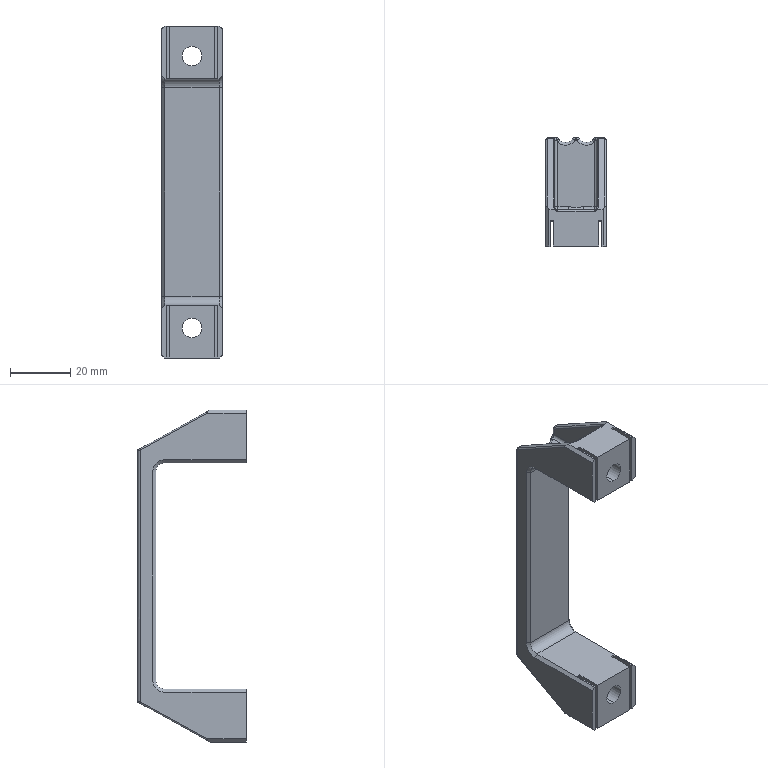Part | SolidWorks | features MBimport 1 | 1 solid | 171 faces | box 20 x 36 x 110 mm | volume 17645 mm3 | plane 56 | cylinder 50 | spline 28 | cone 13 | torus 12 | sphere 12 | commonest cylinder face diameters 2 x24 1 x14 6 x4 6.5 x4 12 x4